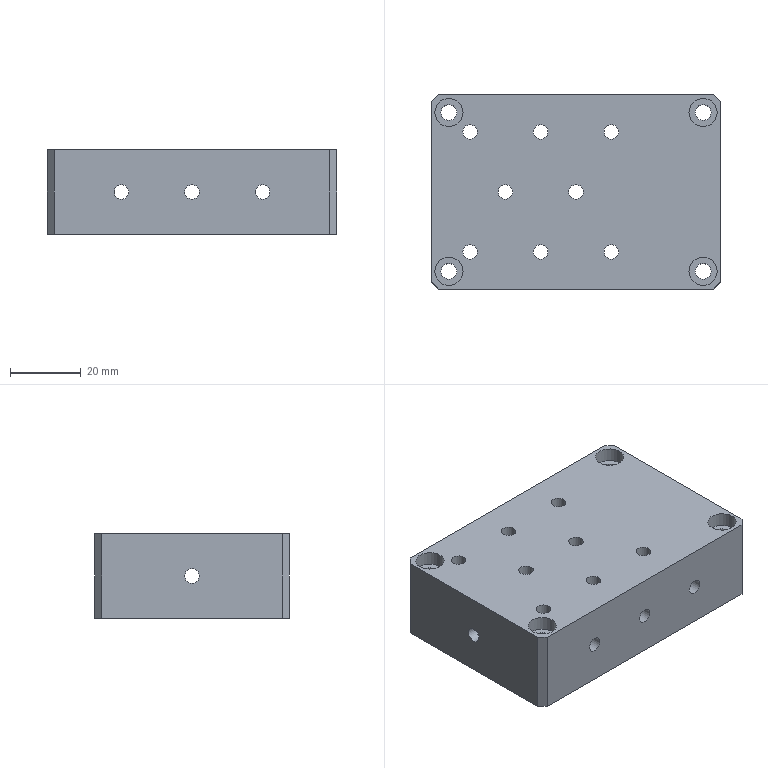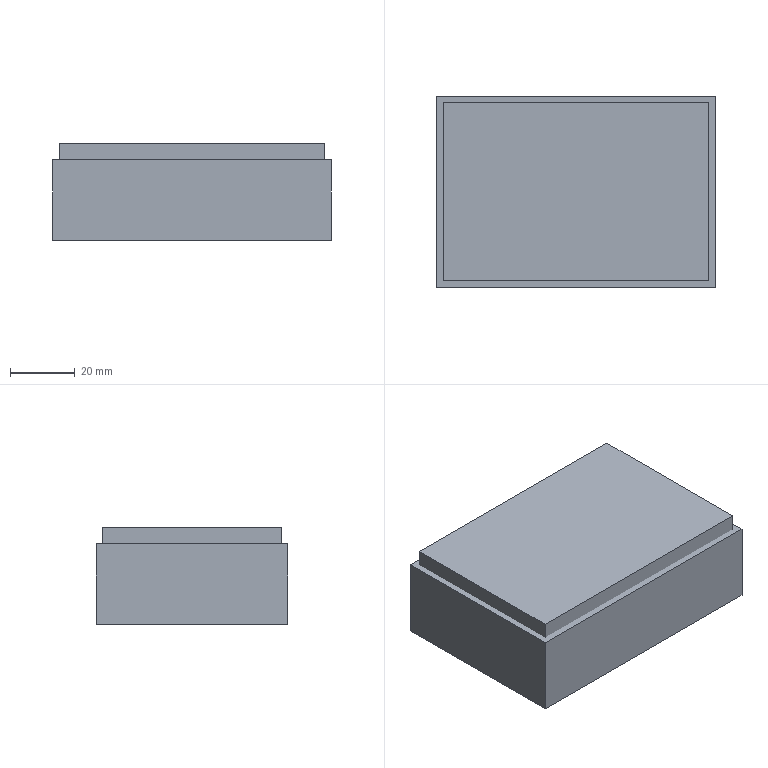CAM job | NX | 3+2 milling, drilling | part box 82 x 55 x 24 mm | stock box 86 x 59 x 30 mm
Tools:
number,name,description,diameter,corner_radius,flute_length,length,flutes
19,D80,Milling Tool-5 Parameters,80.0,0.0,50.0,75.0,2
1,D6A45,Milling Tool-5 Parameters,6.0,0.0,50.0,75.0,2
4,4.2ZT,Drilling Tool,4.1,0.0,35.0,50.0,2
8,4.5ZT,Drilling Tool,4.5,0.0,35.0,50.0,2
15,D10,Milling Tool-5 Parameters,10.0,0.0,50.0,75.0,2
14,D10JING,Milling Tool-5 Parameters,10.0,0.0,50.0,75.0,2
12,D6,Milling Tool-5 Parameters,6.0,0.0,50.0,75.0,2
16,D1.5,Milling Tool-5 Parameters,1.5,0.0,50.0,75.0,2
Operations:
program,operation,operation_type,tool,method,geometry_group,spindle_rpm,surface_speed,feed_per_tooth,feed_cut,feed_plunge,cut_length_mm,path_length_mm,cut_time_min,machine_time_min
1,FLOOR_WALL,VolumeBased25DMillingOperation,D80,METHOD,A,6500.0,1633.0,0.1154,1500.0,100.0,178.0,232.0,0.1187,0.1241
1,DRILLING,Operation,D6A45,METHOD,A,5000.0,94.0,0.035,350.0,0.0,48.0,413.349,0.1371,0.1737
1,DRILLING_COPY_COPY,Operation,4.2ZT,METHOD,A,2000.0,26.0,0.075,300.0,0.0,101.854,425.179,0.3395,0.3718
1,DRILLING_COPY_COPY_COPY,Operation,4.5ZT,METHOD,A,2000.0,26.0,0.075,300.0,0.0,117.408,466.078,0.3914,0.4262
1,ZLEVEL_PROFILE,ZLevelMilling,D10,METHOD,A,9500.0,298.0,0.1579,3000.0,1000.0,7582.959,7663.959,2.559,2.568
1,ZLEVEL_PROFILE_COPY_1,ZLevelMilling,D10JING,METHOD,A,9500.0,298.0,0.0632,1200.0,1000.0,789.466,870.466,0.7391,0.7472
1,HOLE_MILLING,CylinderMilling,D6,METHOD,A,9500.0,179.0,0.0789,1500.0,100.0,264.609,680.609,0.1764,0.218
1,PLANAR_MILL_COPY_COPY_COPY,PlanarMilling,D6A45,METHOD,A,9500.0,179.0,0.0658,1250.0,100.0,477.767,1489.965,0.3822,0.4834
2,FLOOR_WALL_COPY,VolumeBased25DMillingOperation,D80,METHOD,B,6500.0,1633.0,0.1154,1500.0,100.0,1044.0,2178.001,0.696,0.8094
2,FLOOR_WALL_1,VolumeBased25DMillingOperation,D10,METHOD,B,9500.0,0.0,0.0,3500.0,1000.0,6870.671,7261.46,2.426,2.465
2,FLOOR_WALL_1_COPY,VolumeBased25DMillingOperation,D10,METHOD,B,9500.0,0.0,0.0789,1500.0,1000.0,664.925,752.925,0.4464,0.4552
2,PLANAR_PROFILE,PlanarMilling,D1.5,METHOD,B,9500.0,44.0,0.0605,1150.0,850.0,2458.919,2513.818,2.149,2.154
2,PLANAR_MILL_COPY_COPY_COPY_COPY,PlanarMilling,D6A45,METHOD,B,9500.0,179.0,0.0658,1250.0,100.0,996.626,1643.23,0.7973,0.862
3,HOLE_MILLING_COPY,CylinderMilling,D6,METHOD,C,9500.0,179.0,0.0789,1500.0,100.0,316.585,384.085,0.2111,0.2178
3,PLANAR_MILL_COPY_COPY_COPY_COPY_1,PlanarMilling,D6A45,METHOD,C,9500.0,179.0,0.0658,1250.0,100.0,37.704,96.704,0.0302,0.0361